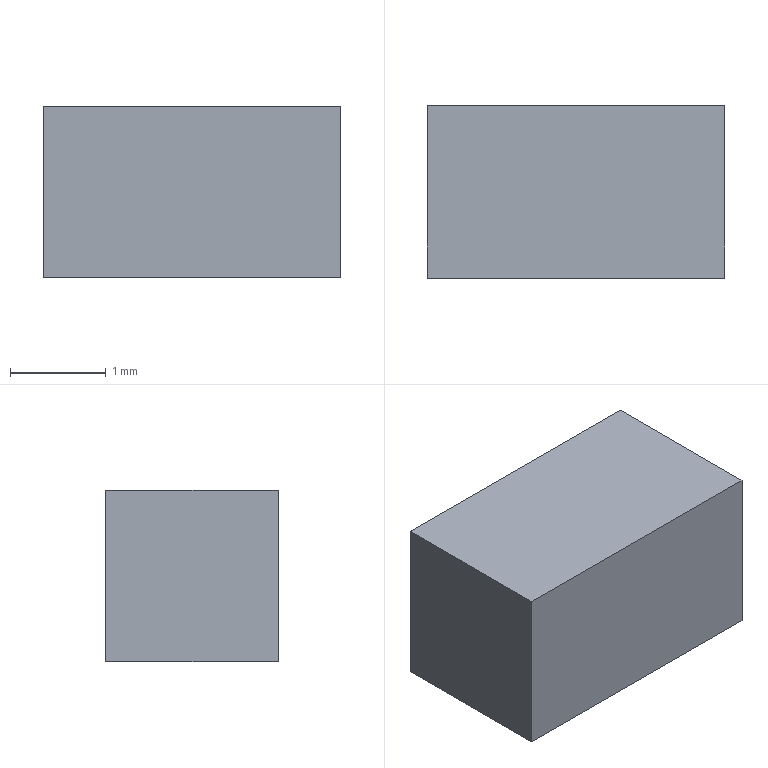Part | Creo | 1 solid | 6 faces | box 3.1 x 1.8 x 1.792 mm | volume 10.001 mm3 | plane 6
STEP:
#1=CARTESIAN_POINT('',(0.,0.,0.));
#2=DIRECTION('',(0.,0.,1.));
#3=DIRECTION('',(1.,0.,0.));
#4=AXIS2_PLACEMENT_3D('',#1,#2,#3);
#5=CARTESIAN_POINT('',(-1.55,0.9,0.));
#6=VERTEX_POINT('',#5);
#7=CARTESIAN_POINT('',(-1.55,-0.9,0.));
#8=VERTEX_POINT('',#7);
#9=CARTESIAN_POINT('',(-1.55,0.9,0.));
#10=DIRECTION('',(0.,-1.,0.));
#11=VECTOR('',#10,1.8);
#12=LINE('',#9,#11);
#13=EDGE_CURVE('',#6,#8,#12,.T.);
#14=ORIENTED_EDGE('',*,*,#13,.T.);
#15=CARTESIAN_POINT('',(1.55,-0.9,0.));
#16=VERTEX_POINT('',#15);
#17=CARTESIAN_POINT('',(-1.55,-0.9,0.));
#18=DIRECTION('',(1.,0.,0.));
#19=VECTOR('',#18,3.1);
#20=LINE('',#17,#19);
#21=EDGE_CURVE('',#8,#16,#20,.T.);
#22=ORIENTED_EDGE('',*,*,#21,.T.);
#23=CARTESIAN_POINT('',(1.55,0.9,0.));
#24=VERTEX_POINT('',#23);
#25=CARTESIAN_POINT('',(1.55,-0.9,0.));
#26=DIRECTION('',(0.,1.,0.));
#27=VECTOR('',#26,1.8);
#28=LINE('',#25,#27);
#29=EDGE_CURVE('',#16,#24,#28,.T.);
#30=ORIENTED_EDGE('',*,*,#29,.T.);
#31=CARTESIAN_POINT('',(1.55,0.9,0.));
#32=DIRECTION('',(-1.,0.,0.));
#33=VECTOR('',#32,3.1);
#34=LINE('',#31,#33);
#35=EDGE_CURVE('',#24,#6,#34,.T.);
#36=ORIENTED_EDGE('',*,*,#35,.T.);
#37=EDGE_LOOP('',(#14,#22,#30,#36));
#38=FACE_OUTER_BOUND('',#37,.F.);
#39=CARTESIAN_POINT('',(0.,0.,0.));
#40=DIRECTION('',(0.,0.,1.));
#41=DIRECTION('',(1.,0.,0.));
#42=AXIS2_PLACEMENT_3D('',#39,#40,#41);
#43=PLANE('',#42);
#44=ADVANCED_FACE('',(#38),#43,.F.);
#45=ORIENTED_EDGE('',*,*,#13,.F.);
#46=CARTESIAN_POINT('',(-1.55,0.9,1.792));
#47=VERTEX_POINT('',#46);
#48=CARTESIAN_POINT('',(-1.55,0.9,0.));
#49=DIRECTION('',(0.,0.,1.));
#50=VECTOR('',#49,1.792);
#51=LINE('',#48,#50);
#52=EDGE_CURVE('',#6,#47,#51,.T.);
#53=ORIENTED_EDGE('',*,*,#52,.T.);
#54=CARTESIAN_POINT('',(-1.55,-0.9,1.792));
#55=VERTEX_POINT('',#54);
#56=CARTESIAN_POINT('',(-1.55,0.9,1.792));
#57=DIRECTION('',(0.,-1.,0.));
#58=VECTOR('',#57,1.8);
#59=LINE('',#56,#58);
#60=EDGE_CURVE('',#47,#55,#59,.T.);
#61=ORIENTED_EDGE('',*,*,#60,.T.);
#62=CARTESIAN_POINT('',(-1.55,-0.9,0.));
#63=DIRECTION('',(0.,0.,1.));
#64=VECTOR('',#63,1.792);
#65=LINE('',#62,#64);
#66=EDGE_CURVE('',#8,#55,#65,.T.);
#67=ORIENTED_EDGE('',*,*,#66,.F.);
#68=EDGE_LOOP('',(#45,#53,#61,#67));
#69=FACE_OUTER_BOUND('',#68,.F.);
#70=CARTESIAN_POINT('',(-1.55,0.9,0.));
#71=DIRECTION('',(-1.,0.,0.));
#72=DIRECTION('',(0.,-1.,0.));
#73=AXIS2_PLACEMENT_3D('',#70,#71,#72);
#74=PLANE('',#73);
#75=ADVANCED_FACE('',(#69),#74,.T.);
#76=ORIENTED_EDGE('',*,*,#35,.F.);
#77=CARTESIAN_POINT('',(1.55,0.9,1.792));
#78=VERTEX_POINT('',#77);
#79=CARTESIAN_POINT('',(1.55,0.9,0.));
#80=DIRECTION('',(0.,0.,1.));
#81=VECTOR('',#80,1.792);
#82=LINE('',#79,#81);
#83=EDGE_CURVE('',#24,#78,#82,.T.);
#84=ORIENTED_EDGE('',*,*,#83,.T.);
#85=CARTESIAN_POINT('',(1.55,0.9,1.792));
#86=DIRECTION('',(-1.,0.,0.));
#87=VECTOR('',#86,3.1);
#88=LINE('',#85,#87);
#89=EDGE_CURVE('',#78,#47,#88,.T.);
#90=ORIENTED_EDGE('',*,*,#89,.T.);
#91=ORIENTED_EDGE('',*,*,#52,.F.);
#92=EDGE_LOOP('',(#76,#84,#90,#91));
#93=FACE_OUTER_BOUND('',#92,.F.);
#94=CARTESIAN_POINT('',(1.55,0.9,0.));
#95=DIRECTION('',(0.,1.,0.));
#96=DIRECTION('',(-1.,0.,0.));
#97=AXIS2_PLACEMENT_3D('',#94,#95,#96);
#98=PLANE('',#97);
#99=ADVANCED_FACE('',(#93),#98,.T.);
#100=ORIENTED_EDGE('',*,*,#29,.F.);
#101=CARTESIAN_POINT('',(1.55,-0.9,1.792));
#102=VERTEX_POINT('',#101);
#103=CARTESIAN_POINT('',(1.55,-0.9,0.));
#104=DIRECTION('',(0.,0.,1.));
#105=VECTOR('',#104,1.792);
#106=LINE('',#103,#105);
#107=EDGE_CURVE('',#16,#102,#106,.T.);
#108=ORIENTED_EDGE('',*,*,#107,.T.);
#109=CARTESIAN_POINT('',(1.55,-0.9,1.792));
#110=DIRECTION('',(0.,1.,0.));
#111=VECTOR('',#110,1.8);
#112=LINE('',#109,#111);
#113=EDGE_CURVE('',#102,#78,#112,.T.);
#114=ORIENTED_EDGE('',*,*,#113,.T.);
#115=ORIENTED_EDGE('',*,*,#83,.F.);
#116=EDGE_LOOP('',(#100,#108,#114,#115));
#117=FACE_OUTER_BOUND('',#116,.F.);
#118=CARTESIAN_POINT('',(1.55,-0.9,0.));
#119=DIRECTION('',(1.,0.,0.));
#120=DIRECTION('',(0.,1.,0.));
#121=AXIS2_PLACEMENT_3D('',#118,#119,#120);
#122=PLANE('',#121);
#123=ADVANCED_FACE('',(#117),#122,.T.);
#124=ORIENTED_EDGE('',*,*,#21,.F.);
#125=ORIENTED_EDGE('',*,*,#66,.T.);
#126=CARTESIAN_POINT('',(-1.55,-0.9,1.792));
#127=DIRECTION('',(1.,0.,0.));
#128=VECTOR('',#127,3.1);
#129=LINE('',#126,#128);
#130=EDGE_CURVE('',#55,#102,#129,.T.);
#131=ORIENTED_EDGE('',*,*,#130,.T.);
#132=ORIENTED_EDGE('',*,*,#107,.F.);
#133=EDGE_LOOP('',(#124,#125,#131,#132));
#134=FACE_OUTER_BOUND('',#133,.F.);
#135=CARTESIAN_POINT('',(-1.55,-0.9,0.));
#136=DIRECTION('',(0.,-1.,0.));
#137=DIRECTION('',(1.,0.,0.));
#138=AXIS2_PLACEMENT_3D('',#135,#136,#137);
#139=PLANE('',#138);
#140=ADVANCED_FACE('',(#134),#139,.T.);
#141=ORIENTED_EDGE('',*,*,#60,.F.);
#142=ORIENTED_EDGE('',*,*,#89,.F.);
#143=ORIENTED_EDGE('',*,*,#113,.F.);
#144=ORIENTED_EDGE('',*,*,#130,.F.);
#145=EDGE_LOOP('',(#141,#142,#143,#144));
#146=FACE_OUTER_BOUND('',#145,.F.);
#147=CARTESIAN_POINT('',(0.,0.,1.792));
#148=DIRECTION('',(0.,0.,1.));
#149=DIRECTION('',(1.,0.,0.));
#150=AXIS2_PLACEMENT_3D('',#147,#148,#149);
#151=PLANE('',#150);
#152=ADVANCED_FACE('',(#146),#151,.T.);
#153=CLOSED_SHELL('',(#44,#75,#99,#123,#140,#152));
#154=MANIFOLD_SOLID_BREP('',#153);
#155=(LENGTH_UNIT()NAMED_UNIT(*)SI_UNIT(.MILLI.,.METRE.));
#156=UNCERTAINTY_MEASURE_WITH_UNIT(LENGTH_MEASURE(0.0004008),#155,'','');
#157=(NAMED_UNIT(*)PLANE_ANGLE_UNIT()SI_UNIT($,.RADIAN.));
#158=PLANE_ANGLE_MEASURE_WITH_UNIT(PLANE_ANGLE_MEASURE(0.01745),#157);
#159=(CONVERSION_BASED_UNIT('DEGREE',#158)NAMED_UNIT(*)PLANE_ANGLE_UNIT());
#160=(NAMED_UNIT(*)SI_UNIT($,.STERADIAN.)SOLID_ANGLE_UNIT());
#161=(GEOMETRIC_REPRESENTATION_CONTEXT(3)GLOBAL_UNCERTAINTY_ASSIGNED_CONTEXT((#156))GLOBAL_UNIT_ASSIGNED_CONTEXT((#155,#159,#160))REPRESENTATION_CONTEXT('',''));
#162=ADVANCED_BREP_SHAPE_REPRESENTATION('',(#4,#154),#161);